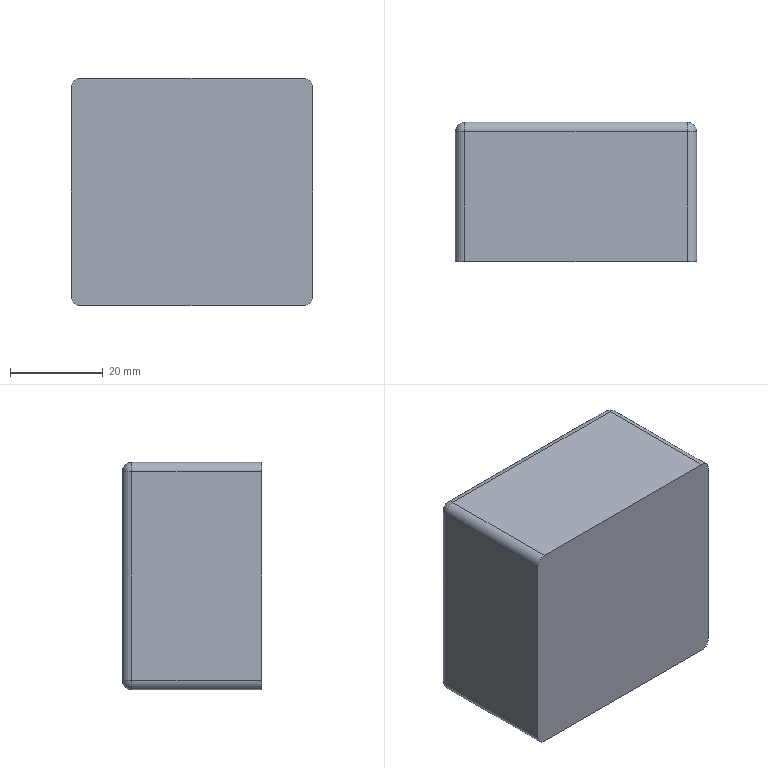Part | NX | 1 solid | 18 faces | box 52 x 30 x 49 mm | volume 76169 mm3 | cylinder 8 | plane 6 | sphere 4 | commonest cylinder face diameters 4 x8
STEP:
#1=CARTESIAN_POINT('',(612.506,-754.5,-862.749));
#2=VERTEX_POINT('',#1);
#3=CARTESIAN_POINT('',(612.506,-782.5,-862.749));
#4=VERTEX_POINT('',#3);
#5=CARTESIAN_POINT('',(612.506,-782.5,-862.749));
#6=DIRECTION('',(0.,-1.,0.));
#7=VECTOR('',#6,1000.);
#8=LINE('',#5,#7);
#9=EDGE_CURVE('',#2,#4,#8,.T.);
#10=ORIENTED_EDGE('',*,*,#9,.F.);
#11=CARTESIAN_POINT('',(612.506,-754.5,-817.749));
#12=VERTEX_POINT('',#11);
#13=CARTESIAN_POINT('',(612.506,-754.5,-726.749));
#14=DIRECTION('',(0.,0.,-1.));
#15=VECTOR('',#14,1000.);
#16=LINE('',#13,#15);
#17=EDGE_CURVE('',#12,#2,#16,.T.);
#18=ORIENTED_EDGE('',*,*,#17,.F.);
#19=CARTESIAN_POINT('',(612.506,-782.5,-817.749));
#20=VERTEX_POINT('',#19);
#21=CARTESIAN_POINT('',(612.506,-782.5,-817.749));
#22=DIRECTION('',(0.,1.,0.));
#23=VECTOR('',#22,1000.);
#24=LINE('',#21,#23);
#25=EDGE_CURVE('',#20,#12,#24,.T.);
#26=ORIENTED_EDGE('',*,*,#25,.F.);
#27=CARTESIAN_POINT('',(612.506,-782.5,-726.749));
#28=DIRECTION('',(0.,0.,-1.));
#29=VECTOR('',#28,1000.);
#30=LINE('',#27,#29);
#31=EDGE_CURVE('',#20,#4,#30,.T.);
#32=ORIENTED_EDGE('',*,*,#31,.T.);
#33=EDGE_LOOP('',(#10,#18,#26,#32));
#34=FACE_BOUND('',#33,.T.);
#35=CARTESIAN_POINT('',(612.506,-782.5,-864.749));
#36=DIRECTION('',(1.,0.,0.));
#37=DIRECTION('',(0.,1.,0.));
#38=AXIS2_PLACEMENT_3D('',#35,#36,#37);
#39=PLANE('',#38);
#40=ADVANCED_FACE('',(#34),#39,.T.);
#41=CARTESIAN_POINT('',(562.506,-782.5,-864.749));
#42=VERTEX_POINT('',#41);
#43=CARTESIAN_POINT('',(562.506,-754.5,-864.749));
#44=VERTEX_POINT('',#43);
#45=CARTESIAN_POINT('',(562.506,-782.5,-864.749));
#46=DIRECTION('',(0.,1.,0.));
#47=VECTOR('',#46,1000.);
#48=LINE('',#45,#47);
#49=EDGE_CURVE('',#42,#44,#48,.T.);
#50=ORIENTED_EDGE('',*,*,#49,.T.);
#51=CARTESIAN_POINT('',(610.506,-754.5,-864.749));
#52=VERTEX_POINT('',#51);
#53=CARTESIAN_POINT('',(692.506,-754.5,-864.749));
#54=DIRECTION('',(1.,0.,0.));
#55=VECTOR('',#54,1000.);
#56=LINE('',#53,#55);
#57=EDGE_CURVE('',#44,#52,#56,.T.);
#58=ORIENTED_EDGE('',*,*,#57,.T.);
#59=CARTESIAN_POINT('',(610.506,-782.5,-864.749));
#60=VERTEX_POINT('',#59);
#61=CARTESIAN_POINT('',(610.506,-782.5,-864.749));
#62=DIRECTION('',(0.,-1.,0.));
#63=VECTOR('',#62,1000.);
#64=LINE('',#61,#63);
#65=EDGE_CURVE('',#52,#60,#64,.T.);
#66=ORIENTED_EDGE('',*,*,#65,.T.);
#67=CARTESIAN_POINT('',(692.506,-782.5,-864.749));
#68=DIRECTION('',(1.,0.,0.));
#69=VECTOR('',#68,1000.);
#70=LINE('',#67,#69);
#71=EDGE_CURVE('',#42,#60,#70,.T.);
#72=ORIENTED_EDGE('',*,*,#71,.F.);
#73=EDGE_LOOP('',(#50,#58,#66,#72));
#74=FACE_BOUND('',#73,.T.);
#75=CARTESIAN_POINT('',(569.506,-782.5,-864.749));
#76=DIRECTION('',(0.,0.,-1.));
#77=DIRECTION('',(0.,-1.,0.));
#78=AXIS2_PLACEMENT_3D('',#75,#76,#77);
#79=PLANE('',#78);
#80=ADVANCED_FACE('',(#74),#79,.T.);
#81=CARTESIAN_POINT('',(560.506,-754.5,-817.749));
#82=VERTEX_POINT('',#81);
#83=CARTESIAN_POINT('',(560.506,-782.5,-817.749));
#84=VERTEX_POINT('',#83);
#85=CARTESIAN_POINT('',(560.506,-782.5,-817.749));
#86=DIRECTION('',(0.,-1.,0.));
#87=VECTOR('',#86,1000.);
#88=LINE('',#85,#87);
#89=EDGE_CURVE('',#82,#84,#88,.T.);
#90=ORIENTED_EDGE('',*,*,#89,.F.);
#91=CARTESIAN_POINT('',(560.506,-754.5,-862.749));
#92=VERTEX_POINT('',#91);
#93=CARTESIAN_POINT('',(560.506,-754.5,-726.749));
#94=DIRECTION('',(0.,0.,1.));
#95=VECTOR('',#94,1000.);
#96=LINE('',#93,#95);
#97=EDGE_CURVE('',#92,#82,#96,.T.);
#98=ORIENTED_EDGE('',*,*,#97,.F.);
#99=CARTESIAN_POINT('',(560.506,-782.5,-862.749));
#100=VERTEX_POINT('',#99);
#101=CARTESIAN_POINT('',(560.506,-782.5,-862.749));
#102=DIRECTION('',(0.,1.,0.));
#103=VECTOR('',#102,1000.);
#104=LINE('',#101,#103);
#105=EDGE_CURVE('',#100,#92,#104,.T.);
#106=ORIENTED_EDGE('',*,*,#105,.F.);
#107=CARTESIAN_POINT('',(560.506,-782.5,-726.749));
#108=DIRECTION('',(0.,0.,1.));
#109=VECTOR('',#108,1000.);
#110=LINE('',#107,#109);
#111=EDGE_CURVE('',#100,#84,#110,.T.);
#112=ORIENTED_EDGE('',*,*,#111,.T.);
#113=EDGE_LOOP('',(#90,#98,#106,#112));
#114=FACE_BOUND('',#113,.T.);
#115=CARTESIAN_POINT('',(560.506,-782.5,-815.749));
#116=DIRECTION('',(-1.,0.,0.));
#117=DIRECTION('',(0.,0.,1.));
#118=AXIS2_PLACEMENT_3D('',#115,#116,#117);
#119=PLANE('',#118);
#120=ADVANCED_FACE('',(#114),#119,.T.);
#121=CARTESIAN_POINT('',(610.506,-782.5,-815.749));
#122=VERTEX_POINT('',#121);
#123=CARTESIAN_POINT('',(562.506,-782.5,-815.749));
#124=VERTEX_POINT('',#123);
#125=CARTESIAN_POINT('',(692.506,-782.5,-815.749));
#126=DIRECTION('',(-1.,0.,0.));
#127=VECTOR('',#126,1000.);
#128=LINE('',#125,#127);
#129=EDGE_CURVE('',#122,#124,#128,.T.);
#130=ORIENTED_EDGE('',*,*,#129,.F.);
#131=CARTESIAN_POINT('',(610.506,-754.5,-815.749));
#132=VERTEX_POINT('',#131);
#133=CARTESIAN_POINT('',(610.506,-782.5,-815.749));
#134=DIRECTION('',(0.,1.,0.));
#135=VECTOR('',#134,1000.);
#136=LINE('',#133,#135);
#137=EDGE_CURVE('',#122,#132,#136,.T.);
#138=ORIENTED_EDGE('',*,*,#137,.T.);
#139=CARTESIAN_POINT('',(562.506,-754.5,-815.749));
#140=VERTEX_POINT('',#139);
#141=CARTESIAN_POINT('',(692.506,-754.5,-815.749));
#142=DIRECTION('',(1.,0.,0.));
#143=VECTOR('',#142,1000.);
#144=LINE('',#141,#143);
#145=EDGE_CURVE('',#140,#132,#144,.T.);
#146=ORIENTED_EDGE('',*,*,#145,.F.);
#147=CARTESIAN_POINT('',(562.506,-782.5,-815.749));
#148=DIRECTION('',(0.,-1.,0.));
#149=VECTOR('',#148,1000.);
#150=LINE('',#147,#149);
#151=EDGE_CURVE('',#140,#124,#150,.T.);
#152=ORIENTED_EDGE('',*,*,#151,.T.);
#153=EDGE_LOOP('',(#130,#138,#146,#152));
#154=FACE_BOUND('',#153,.T.);
#155=CARTESIAN_POINT('',(603.506,-782.5,-815.749));
#156=DIRECTION('',(0.,0.,1.));
#157=DIRECTION('',(1.,0.,0.));
#158=AXIS2_PLACEMENT_3D('',#155,#156,#157);
#159=PLANE('',#158);
#160=ADVANCED_FACE('',(#154),#159,.T.);
#161=ORIENTED_EDGE('',*,*,#9,.T.);
#162=CARTESIAN_POINT('',(610.506,-782.5,-862.749));
#163=DIRECTION('',(0.,-1.,0.));
#164=DIRECTION('',(1.,0.,0.));
#165=AXIS2_PLACEMENT_3D('',#162,#163,#164);
#166=CIRCLE('',#165,2.);
#167=EDGE_CURVE('',#60,#4,#166,.T.);
#168=ORIENTED_EDGE('',*,*,#167,.F.);
#169=ORIENTED_EDGE('',*,*,#65,.F.);
#170=CARTESIAN_POINT('',(610.506,-754.5,-862.749));
#171=DIRECTION('',(0.,-1.,0.));
#172=DIRECTION('',(-1.,0.,0.));
#173=AXIS2_PLACEMENT_3D('',#170,#171,#172);
#174=CIRCLE('',#173,2.);
#175=EDGE_CURVE('',#52,#2,#174,.T.);
#176=ORIENTED_EDGE('',*,*,#175,.T.);
#177=EDGE_LOOP('',(#161,#168,#169,#176));
#178=FACE_BOUND('',#177,.T.);
#179=CARTESIAN_POINT('',(610.506,-782.5,-862.749));
#180=DIRECTION('',(0.,-1.,0.));
#181=DIRECTION('',(1.,0.,0.));
#182=AXIS2_PLACEMENT_3D('',#179,#180,#181);
#183=CYLINDRICAL_SURFACE('',#182,2.);
#184=ADVANCED_FACE('',(#178),#183,.T.);
#185=ORIENTED_EDGE('',*,*,#49,.F.);
#186=CARTESIAN_POINT('',(562.506,-782.5,-862.749));
#187=DIRECTION('',(0.,1.,0.));
#188=DIRECTION('',(-1.,0.,0.));
#189=AXIS2_PLACEMENT_3D('',#186,#187,#188);
#190=CIRCLE('',#189,2.);
#191=EDGE_CURVE('',#42,#100,#190,.T.);
#192=ORIENTED_EDGE('',*,*,#191,.T.);
#193=ORIENTED_EDGE('',*,*,#105,.T.);
#194=CARTESIAN_POINT('',(562.506,-754.5,-862.749));
#195=DIRECTION('',(0.,1.,0.));
#196=DIRECTION('',(-1.,0.,0.));
#197=AXIS2_PLACEMENT_3D('',#194,#195,#196);
#198=CIRCLE('',#197,2.);
#199=EDGE_CURVE('',#44,#92,#198,.T.);
#200=ORIENTED_EDGE('',*,*,#199,.F.);
#201=EDGE_LOOP('',(#185,#192,#193,#200));
#202=FACE_BOUND('',#201,.T.);
#203=CARTESIAN_POINT('',(562.506,-782.5,-862.749));
#204=DIRECTION('',(0.,1.,0.));
#205=DIRECTION('',(-1.,0.,0.));
#206=AXIS2_PLACEMENT_3D('',#203,#204,#205);
#207=CYLINDRICAL_SURFACE('',#206,2.);
#208=ADVANCED_FACE('',(#202),#207,.T.);
#209=CARTESIAN_POINT('',(610.506,-754.5,-817.749));
#210=DIRECTION('',(0.,-1.,0.));
#211=DIRECTION('',(-1.,0.,0.));
#212=AXIS2_PLACEMENT_3D('',#209,#210,#211);
#213=CIRCLE('',#212,2.);
#214=EDGE_CURVE('',#12,#132,#213,.T.);
#215=ORIENTED_EDGE('',*,*,#214,.T.);
#216=ORIENTED_EDGE('',*,*,#137,.F.);
#217=CARTESIAN_POINT('',(610.506,-782.5,-817.749));
#218=DIRECTION('',(0.,1.,0.));
#219=DIRECTION('',(-1.,0.,0.));
#220=AXIS2_PLACEMENT_3D('',#217,#218,#219);
#221=CIRCLE('',#220,2.);
#222=EDGE_CURVE('',#122,#20,#221,.T.);
#223=ORIENTED_EDGE('',*,*,#222,.T.);
#224=ORIENTED_EDGE('',*,*,#25,.T.);
#225=EDGE_LOOP('',(#215,#216,#223,#224));
#226=FACE_BOUND('',#225,.T.);
#227=CARTESIAN_POINT('',(610.506,-782.5,-817.749));
#228=DIRECTION('',(0.,1.,0.));
#229=DIRECTION('',(-1.,0.,0.));
#230=AXIS2_PLACEMENT_3D('',#227,#228,#229);
#231=CYLINDRICAL_SURFACE('',#230,2.);
#232=ADVANCED_FACE('',(#226),#231,.T.);
#233=ORIENTED_EDGE('',*,*,#89,.T.);
#234=CARTESIAN_POINT('',(562.506,-782.5,-817.749));
#235=DIRECTION('',(0.,-1.,0.));
#236=DIRECTION('',(1.,0.,0.));
#237=AXIS2_PLACEMENT_3D('',#234,#235,#236);
#238=CIRCLE('',#237,2.);
#239=EDGE_CURVE('',#124,#84,#238,.T.);
#240=ORIENTED_EDGE('',*,*,#239,.F.);
#241=ORIENTED_EDGE('',*,*,#151,.F.);
#242=CARTESIAN_POINT('',(562.506,-754.5,-817.749));
#243=DIRECTION('',(0.,-1.,0.));
#244=DIRECTION('',(1.,0.,0.));
#245=AXIS2_PLACEMENT_3D('',#242,#243,#244);
#246=CIRCLE('',#245,2.);
#247=EDGE_CURVE('',#140,#82,#246,.T.);
#248=ORIENTED_EDGE('',*,*,#247,.T.);
#249=EDGE_LOOP('',(#233,#240,#241,#248));
#250=FACE_BOUND('',#249,.T.);
#251=CARTESIAN_POINT('',(562.506,-782.5,-817.749));
#252=DIRECTION('',(0.,-1.,0.));
#253=DIRECTION('',(1.,0.,0.));
#254=AXIS2_PLACEMENT_3D('',#251,#252,#253);
#255=CYLINDRICAL_SURFACE('',#254,2.);
#256=ADVANCED_FACE('',(#250),#255,.T.);
#257=ORIENTED_EDGE('',*,*,#214,.F.);
#258=CARTESIAN_POINT('',(610.506,-752.5,-817.749));
#259=VERTEX_POINT('',#258);
#260=CARTESIAN_POINT('',(610.506,-754.5,-817.749));
#261=DIRECTION('',(0.,0.,-1.));
#262=DIRECTION('',(1.,0.,0.));
#263=AXIS2_PLACEMENT_3D('',#260,#261,#262);
#264=CIRCLE('',#263,2.);
#265=EDGE_CURVE('',#259,#12,#264,.T.);
#266=ORIENTED_EDGE('',*,*,#265,.F.);
#267=CARTESIAN_POINT('',(610.506,-754.5,-817.749));
#268=DIRECTION('',(1.,0.,0.));
#269=DIRECTION('',(0.,0.,1.));
#270=AXIS2_PLACEMENT_3D('',#267,#268,#269);
#271=CIRCLE('',#270,2.);
#272=EDGE_CURVE('',#259,#132,#271,.T.);
#273=ORIENTED_EDGE('',*,*,#272,.T.);
#274=EDGE_LOOP('',(#257,#266,#273));
#275=FACE_BOUND('',#274,.T.);
#276=CARTESIAN_POINT('',(610.506,-754.5,-817.749));
#277=DIRECTION('',(0.,-1.,0.));
#278=DIRECTION('',(-1.,0.,0.));
#279=AXIS2_PLACEMENT_3D('',#276,#277,#278);
#280=SPHERICAL_SURFACE('',#279,2.);
#281=ADVANCED_FACE('',(#275),#280,.T.);
#282=CARTESIAN_POINT('',(562.506,-752.5,-862.749));
#283=VERTEX_POINT('',#282);
#284=CARTESIAN_POINT('',(610.506,-752.5,-862.749));
#285=VERTEX_POINT('',#284);
#286=CARTESIAN_POINT('',(692.506,-752.5,-862.749));
#287=DIRECTION('',(1.,0.,0.));
#288=VECTOR('',#287,1000.);
#289=LINE('',#286,#288);
#290=EDGE_CURVE('',#283,#285,#289,.T.);
#291=ORIENTED_EDGE('',*,*,#290,.F.);
#292=CARTESIAN_POINT('',(562.506,-752.5,-817.749));
#293=VERTEX_POINT('',#292);
#294=CARTESIAN_POINT('',(562.506,-752.5,-726.749));
#295=DIRECTION('',(0.,0.,1.));
#296=VECTOR('',#295,1000.);
#297=LINE('',#294,#296);
#298=EDGE_CURVE('',#283,#293,#297,.T.);
#299=ORIENTED_EDGE('',*,*,#298,.T.);
#300=CARTESIAN_POINT('',(692.506,-752.5,-817.749));
#301=DIRECTION('',(1.,0.,0.));
#302=VECTOR('',#301,1000.);
#303=LINE('',#300,#302);
#304=EDGE_CURVE('',#293,#259,#303,.T.);
#305=ORIENTED_EDGE('',*,*,#304,.T.);
#306=CARTESIAN_POINT('',(610.506,-752.5,-726.749));
#307=DIRECTION('',(0.,0.,-1.));
#308=VECTOR('',#307,1000.);
#309=LINE('',#306,#308);
#310=EDGE_CURVE('',#259,#285,#309,.T.);
#311=ORIENTED_EDGE('',*,*,#310,.T.);
#312=EDGE_LOOP('',(#291,#299,#305,#311));
#313=FACE_BOUND('',#312,.T.);
#314=CARTESIAN_POINT('',(692.506,-752.5,-726.749));
#315=DIRECTION('',(0.,1.,0.));
#316=DIRECTION('',(1.,0.,0.));
#317=AXIS2_PLACEMENT_3D('',#314,#315,#316);
#318=PLANE('',#317);
#319=ADVANCED_FACE('',(#313),#318,.T.);
#320=CARTESIAN_POINT('',(610.506,-754.5,-862.749));
#321=DIRECTION('',(-1.,0.,0.));
#322=DIRECTION('',(0.,0.,-1.));
#323=AXIS2_PLACEMENT_3D('',#320,#321,#322);
#324=CIRCLE('',#323,2.);
#325=EDGE_CURVE('',#285,#52,#324,.T.);
#326=ORIENTED_EDGE('',*,*,#325,.T.);
#327=ORIENTED_EDGE('',*,*,#57,.F.);
#328=CARTESIAN_POINT('',(562.506,-754.5,-862.749));
#329=DIRECTION('',(-1.,0.,0.));
#330=DIRECTION('',(0.,0.,-1.));
#331=AXIS2_PLACEMENT_3D('',#328,#329,#330);
#332=CIRCLE('',#331,2.);
#333=EDGE_CURVE('',#283,#44,#332,.T.);
#334=ORIENTED_EDGE('',*,*,#333,.F.);
#335=ORIENTED_EDGE('',*,*,#290,.T.);
#336=EDGE_LOOP('',(#326,#327,#334,#335));
#337=FACE_BOUND('',#336,.T.);
#338=CARTESIAN_POINT('',(692.506,-754.5,-862.749));
#339=DIRECTION('',(1.,0.,0.));
#340=DIRECTION('',(0.,0.,1.));
#341=AXIS2_PLACEMENT_3D('',#338,#339,#340);
#342=CYLINDRICAL_SURFACE('',#341,2.);
#343=ADVANCED_FACE('',(#337),#342,.T.);
#344=CARTESIAN_POINT('',(562.506,-754.5,-817.749));
#345=DIRECTION('',(0.,0.,1.));
#346=DIRECTION('',(-1.,0.,0.));
#347=AXIS2_PLACEMENT_3D('',#344,#345,#346);
#348=CIRCLE('',#347,2.);
#349=EDGE_CURVE('',#293,#82,#348,.T.);
#350=ORIENTED_EDGE('',*,*,#349,.F.);
#351=ORIENTED_EDGE('',*,*,#298,.F.);
#352=CARTESIAN_POINT('',(562.506,-754.5,-862.749));
#353=DIRECTION('',(0.,0.,1.));
#354=DIRECTION('',(-1.,0.,0.));
#355=AXIS2_PLACEMENT_3D('',#352,#353,#354);
#356=CIRCLE('',#355,2.);
#357=EDGE_CURVE('',#283,#92,#356,.T.);
#358=ORIENTED_EDGE('',*,*,#357,.T.);
#359=ORIENTED_EDGE('',*,*,#97,.T.);
#360=EDGE_LOOP('',(#350,#351,#358,#359));
#361=FACE_BOUND('',#360,.T.);
#362=CARTESIAN_POINT('',(562.506,-754.5,-726.749));
#363=DIRECTION('',(0.,0.,1.));
#364=DIRECTION('',(-1.,0.,0.));
#365=AXIS2_PLACEMENT_3D('',#362,#363,#364);
#366=CYLINDRICAL_SURFACE('',#365,2.);
#367=ADVANCED_FACE('',(#361),#366,.T.);
#368=ORIENTED_EDGE('',*,*,#333,.T.);
#369=ORIENTED_EDGE('',*,*,#199,.T.);
#370=ORIENTED_EDGE('',*,*,#357,.F.);
#371=EDGE_LOOP('',(#368,#369,#370));
#372=FACE_BOUND('',#371,.T.);
#373=CARTESIAN_POINT('',(562.506,-754.5,-862.749));
#374=DIRECTION('',(0.,0.,1.));
#375=DIRECTION('',(-1.,0.,0.));
#376=AXIS2_PLACEMENT_3D('',#373,#374,#375);
#377=SPHERICAL_SURFACE('',#376,2.);
#378=ADVANCED_FACE('',(#372),#377,.T.);
#379=ORIENTED_EDGE('',*,*,#325,.F.);
#380=CARTESIAN_POINT('',(610.506,-754.5,-862.749));
#381=DIRECTION('',(0.,0.,-1.));
#382=DIRECTION('',(1.,0.,0.));
#383=AXIS2_PLACEMENT_3D('',#380,#381,#382);
#384=CIRCLE('',#383,2.);
#385=EDGE_CURVE('',#285,#2,#384,.T.);
#386=ORIENTED_EDGE('',*,*,#385,.T.);
#387=ORIENTED_EDGE('',*,*,#175,.F.);
#388=EDGE_LOOP('',(#379,#386,#387));
#389=FACE_BOUND('',#388,.T.);
#390=CARTESIAN_POINT('',(610.506,-754.5,-862.749));
#391=DIRECTION('',(0.,-1.,0.));
#392=DIRECTION('',(1.,0.,0.));
#393=AXIS2_PLACEMENT_3D('',#390,#391,#392);
#394=SPHERICAL_SURFACE('',#393,2.);
#395=ADVANCED_FACE('',(#389),#394,.T.);
#396=ORIENTED_EDGE('',*,*,#349,.T.);
#397=ORIENTED_EDGE('',*,*,#247,.F.);
#398=CARTESIAN_POINT('',(562.506,-754.5,-817.749));
#399=DIRECTION('',(1.,0.,0.));
#400=DIRECTION('',(0.,0.,1.));
#401=AXIS2_PLACEMENT_3D('',#398,#399,#400);
#402=CIRCLE('',#401,2.);
#403=EDGE_CURVE('',#293,#140,#402,.T.);
#404=ORIENTED_EDGE('',*,*,#403,.F.);
#405=EDGE_LOOP('',(#396,#397,#404));
#406=FACE_BOUND('',#405,.T.);
#407=CARTESIAN_POINT('',(562.506,-754.5,-817.749));
#408=DIRECTION('',(0.,0.,1.));
#409=DIRECTION('',(-1.,0.,0.));
#410=AXIS2_PLACEMENT_3D('',#407,#408,#409);
#411=SPHERICAL_SURFACE('',#410,2.);
#412=ADVANCED_FACE('',(#406),#411,.T.);
#413=ORIENTED_EDGE('',*,*,#304,.F.);
#414=ORIENTED_EDGE('',*,*,#403,.T.);
#415=ORIENTED_EDGE('',*,*,#145,.T.);
#416=ORIENTED_EDGE('',*,*,#272,.F.);
#417=EDGE_LOOP('',(#413,#414,#415,#416));
#418=FACE_BOUND('',#417,.T.);
#419=CARTESIAN_POINT('',(692.506,-754.5,-817.749));
#420=DIRECTION('',(1.,0.,0.));
#421=DIRECTION('',(0.,0.,1.));
#422=AXIS2_PLACEMENT_3D('',#419,#420,#421);
#423=CYLINDRICAL_SURFACE('',#422,2.);
#424=ADVANCED_FACE('',(#418),#423,.T.);
#425=ORIENTED_EDGE('',*,*,#310,.F.);
#426=ORIENTED_EDGE('',*,*,#265,.T.);
#427=ORIENTED_EDGE('',*,*,#17,.T.);
#428=ORIENTED_EDGE('',*,*,#385,.F.);
#429=EDGE_LOOP('',(#425,#426,#427,#428));
#430=FACE_BOUND('',#429,.T.);
#431=CARTESIAN_POINT('',(610.506,-754.5,-726.749));
#432=DIRECTION('',(0.,0.,-1.));
#433=DIRECTION('',(1.,0.,0.));
#434=AXIS2_PLACEMENT_3D('',#431,#432,#433);
#435=CYLINDRICAL_SURFACE('',#434,2.);
#436=ADVANCED_FACE('',(#430),#435,.T.);
#437=ORIENTED_EDGE('',*,*,#129,.T.);
#438=ORIENTED_EDGE('',*,*,#239,.T.);
#439=ORIENTED_EDGE('',*,*,#111,.F.);
#440=ORIENTED_EDGE('',*,*,#191,.F.);
#441=ORIENTED_EDGE('',*,*,#71,.T.);
#442=ORIENTED_EDGE('',*,*,#167,.T.);
#443=ORIENTED_EDGE('',*,*,#31,.F.);
#444=ORIENTED_EDGE('',*,*,#222,.F.);
#445=EDGE_LOOP('',(#437,#438,#439,#440,#441,#442,#443,#444));
#446=FACE_BOUND('',#445,.T.);
#447=CARTESIAN_POINT('',(692.506,-782.5,-726.749));
#448=DIRECTION('',(0.,1.,0.));
#449=DIRECTION('',(1.,0.,0.));
#450=AXIS2_PLACEMENT_3D('',#447,#448,#449);
#451=PLANE('',#450);
#452=ADVANCED_FACE('',(#446),#451,.F.);
#453=CLOSED_SHELL('',(#40,#80,#120,#160,#184,#208,#232,#256,#281,#319,#343,#367,#378,#395,#412,#424,#436,#452));
#454=MANIFOLD_SOLID_BREP('',#453);
#455=(LENGTH_UNIT()NAMED_UNIT(*)SI_UNIT(.MILLI.,.METRE.));
#456=UNCERTAINTY_MEASURE_WITH_UNIT(LENGTH_MEASURE(0.00001),#455,'','');
#457=(NAMED_UNIT(*)PLANE_ANGLE_UNIT()SI_UNIT($,.RADIAN.));
#458=(NAMED_UNIT(*)SI_UNIT($,.STERADIAN.)SOLID_ANGLE_UNIT());
#459=(GEOMETRIC_REPRESENTATION_CONTEXT(3)GLOBAL_UNCERTAINTY_ASSIGNED_CONTEXT((#456))GLOBAL_UNIT_ASSIGNED_CONTEXT((#455,#457,#458))REPRESENTATION_CONTEXT('',''));
#460=ADVANCED_BREP_SHAPE_REPRESENTATION('',(#454),#459);